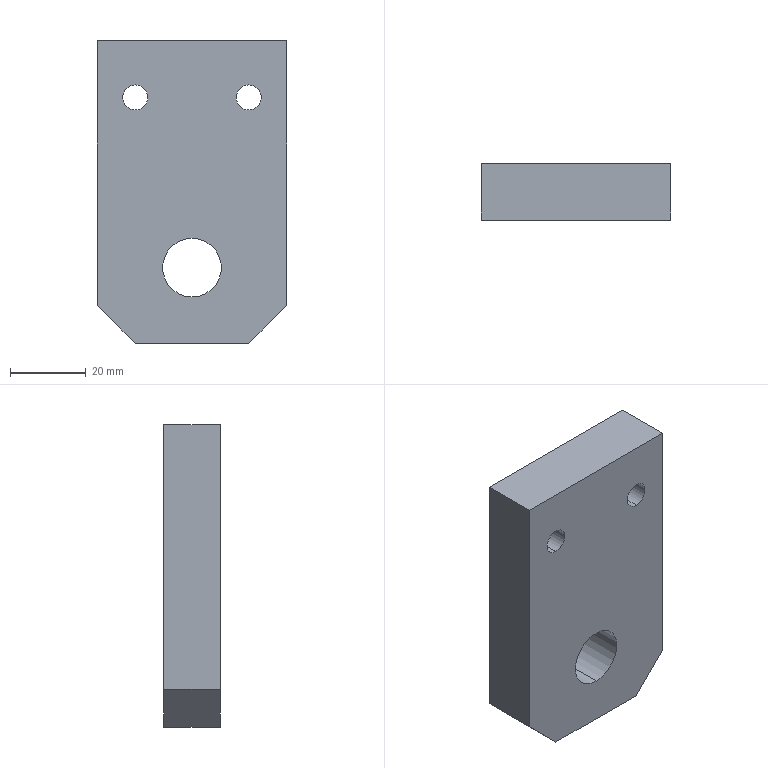Part | SolidWorks | features BaseBody 1 | 1 solid | 20 faces | box 50 x 15 x 80 mm | volume 53816 mm3 | cylinder 10 | plane 10 | commonest cylinder face diameters 6.6 x4 11 x4 15.5 x2
STEP:
#1=CARTESIAN_POINT('',(15.,8.2,-20.5));
#2=VERTEX_POINT('',#1);
#3=CARTESIAN_POINT('',(15.,8.2,-9.5));
#4=VERTEX_POINT('',#3);
#5=CARTESIAN_POINT('',(15.,8.2,-15.));
#6=DIRECTION('',(0.,1.,0.));
#7=DIRECTION('',(0.,0.,1.));
#8=AXIS2_PLACEMENT_3D('',#5,#6,#7);
#9=CIRCLE('',#8,5.5);
#10=EDGE_CURVE('',#2,#4,#9,.T.);
#11=ORIENTED_EDGE('',*,*,#10,.F.);
#12=CARTESIAN_POINT('',(15.,15.,-20.5));
#13=VERTEX_POINT('',#12);
#14=CARTESIAN_POINT('',(15.,15.,-20.5));
#15=DIRECTION('',(0.,1.,0.));
#16=VECTOR('',#15,1000.);
#17=LINE('',#14,#16);
#18=EDGE_CURVE('',#2,#13,#17,.T.);
#19=ORIENTED_EDGE('',*,*,#18,.T.);
#20=CARTESIAN_POINT('',(15.,15.,-9.5));
#21=VERTEX_POINT('',#20);
#22=CARTESIAN_POINT('',(15.,15.,-15.));
#23=DIRECTION('',(0.,1.,0.));
#24=DIRECTION('',(0.,0.,1.));
#25=AXIS2_PLACEMENT_3D('',#22,#23,#24);
#26=CIRCLE('',#25,5.5);
#27=EDGE_CURVE('',#13,#21,#26,.T.);
#28=ORIENTED_EDGE('',*,*,#27,.T.);
#29=CARTESIAN_POINT('',(15.,15.,-9.5));
#30=DIRECTION('',(0.,1.,0.));
#31=VECTOR('',#30,1000.);
#32=LINE('',#29,#31);
#33=EDGE_CURVE('',#4,#21,#32,.T.);
#34=ORIENTED_EDGE('',*,*,#33,.F.);
#35=EDGE_LOOP('',(#11,#19,#28,#34));
#36=FACE_OUTER_BOUND('',#35,.T.);
#37=CARTESIAN_POINT('',(15.,15.,-15.));
#38=DIRECTION('',(0.,1.,0.));
#39=DIRECTION('',(0.,0.,1.));
#40=AXIS2_PLACEMENT_3D('',#37,#38,#39);
#41=CYLINDRICAL_SURFACE('',#40,5.5);
#42=ADVANCED_FACE('',(#36),#41,.F.);
#43=CARTESIAN_POINT('',(15.,0.,-18.3));
#44=VERTEX_POINT('',#43);
#45=CARTESIAN_POINT('',(15.,0.,-11.7));
#46=VERTEX_POINT('',#45);
#47=CARTESIAN_POINT('',(15.,0.,-15.));
#48=DIRECTION('',(0.,1.,0.));
#49=DIRECTION('',(0.,0.,1.));
#50=AXIS2_PLACEMENT_3D('',#47,#48,#49);
#51=CIRCLE('',#50,3.3);
#52=EDGE_CURVE('',#44,#46,#51,.T.);
#53=ORIENTED_EDGE('',*,*,#52,.F.);
#54=CARTESIAN_POINT('',(15.,8.2,-18.3));
#55=VERTEX_POINT('',#54);
#56=CARTESIAN_POINT('',(15.,15.,-18.3));
#57=DIRECTION('',(0.,1.,0.));
#58=VECTOR('',#57,1000.);
#59=LINE('',#56,#58);
#60=EDGE_CURVE('',#44,#55,#59,.T.);
#61=ORIENTED_EDGE('',*,*,#60,.T.);
#62=CARTESIAN_POINT('',(15.,8.2,-11.7));
#63=VERTEX_POINT('',#62);
#64=CARTESIAN_POINT('',(15.,8.2,-15.));
#65=DIRECTION('',(0.,1.,0.));
#66=DIRECTION('',(0.,0.,1.));
#67=AXIS2_PLACEMENT_3D('',#64,#65,#66);
#68=CIRCLE('',#67,3.3);
#69=EDGE_CURVE('',#55,#63,#68,.T.);
#70=ORIENTED_EDGE('',*,*,#69,.T.);
#71=CARTESIAN_POINT('',(15.,15.,-11.7));
#72=DIRECTION('',(0.,1.,0.));
#73=VECTOR('',#72,1000.);
#74=LINE('',#71,#73);
#75=EDGE_CURVE('',#46,#63,#74,.T.);
#76=ORIENTED_EDGE('',*,*,#75,.F.);
#77=EDGE_LOOP('',(#53,#61,#70,#76));
#78=FACE_OUTER_BOUND('',#77,.T.);
#79=CARTESIAN_POINT('',(15.,15.,-15.));
#80=DIRECTION('',(0.,1.,0.));
#81=DIRECTION('',(0.,0.,1.));
#82=AXIS2_PLACEMENT_3D('',#79,#80,#81);
#83=CYLINDRICAL_SURFACE('',#82,3.3);
#84=ADVANCED_FACE('',(#78),#83,.F.);
#85=CARTESIAN_POINT('',(-15.,8.2,-20.5));
#86=VERTEX_POINT('',#85);
#87=CARTESIAN_POINT('',(-15.,8.2,-9.5));
#88=VERTEX_POINT('',#87);
#89=CARTESIAN_POINT('',(-15.,8.2,-15.));
#90=DIRECTION('',(0.,1.,0.));
#91=DIRECTION('',(0.,0.,1.));
#92=AXIS2_PLACEMENT_3D('',#89,#90,#91);
#93=CIRCLE('',#92,5.5);
#94=EDGE_CURVE('',#86,#88,#93,.T.);
#95=ORIENTED_EDGE('',*,*,#94,.F.);
#96=CARTESIAN_POINT('',(-15.,15.,-20.5));
#97=VERTEX_POINT('',#96);
#98=CARTESIAN_POINT('',(-15.,15.,-20.5));
#99=DIRECTION('',(0.,1.,0.));
#100=VECTOR('',#99,1000.);
#101=LINE('',#98,#100);
#102=EDGE_CURVE('',#86,#97,#101,.T.);
#103=ORIENTED_EDGE('',*,*,#102,.T.);
#104=CARTESIAN_POINT('',(-15.,15.,-9.5));
#105=VERTEX_POINT('',#104);
#106=CARTESIAN_POINT('',(-15.,15.,-15.));
#107=DIRECTION('',(0.,1.,0.));
#108=DIRECTION('',(0.,0.,1.));
#109=AXIS2_PLACEMENT_3D('',#106,#107,#108);
#110=CIRCLE('',#109,5.5);
#111=EDGE_CURVE('',#97,#105,#110,.T.);
#112=ORIENTED_EDGE('',*,*,#111,.T.);
#113=CARTESIAN_POINT('',(-15.,15.,-9.5));
#114=DIRECTION('',(0.,1.,0.));
#115=VECTOR('',#114,1000.);
#116=LINE('',#113,#115);
#117=EDGE_CURVE('',#88,#105,#116,.T.);
#118=ORIENTED_EDGE('',*,*,#117,.F.);
#119=EDGE_LOOP('',(#95,#103,#112,#118));
#120=FACE_OUTER_BOUND('',#119,.T.);
#121=CARTESIAN_POINT('',(-15.,15.,-15.));
#122=DIRECTION('',(0.,1.,0.));
#123=DIRECTION('',(0.,0.,1.));
#124=AXIS2_PLACEMENT_3D('',#121,#122,#123);
#125=CYLINDRICAL_SURFACE('',#124,5.5);
#126=ADVANCED_FACE('',(#120),#125,.F.);
#127=CARTESIAN_POINT('',(-15.,0.,-18.3));
#128=VERTEX_POINT('',#127);
#129=CARTESIAN_POINT('',(-15.,0.,-11.7));
#130=VERTEX_POINT('',#129);
#131=CARTESIAN_POINT('',(-15.,0.,-15.));
#132=DIRECTION('',(0.,1.,0.));
#133=DIRECTION('',(0.,0.,1.));
#134=AXIS2_PLACEMENT_3D('',#131,#132,#133);
#135=CIRCLE('',#134,3.3);
#136=EDGE_CURVE('',#128,#130,#135,.T.);
#137=ORIENTED_EDGE('',*,*,#136,.F.);
#138=CARTESIAN_POINT('',(-15.,8.2,-18.3));
#139=VERTEX_POINT('',#138);
#140=CARTESIAN_POINT('',(-15.,15.,-18.3));
#141=DIRECTION('',(0.,1.,0.));
#142=VECTOR('',#141,1000.);
#143=LINE('',#140,#142);
#144=EDGE_CURVE('',#128,#139,#143,.T.);
#145=ORIENTED_EDGE('',*,*,#144,.T.);
#146=CARTESIAN_POINT('',(-15.,8.2,-11.7));
#147=VERTEX_POINT('',#146);
#148=CARTESIAN_POINT('',(-15.,8.2,-15.));
#149=DIRECTION('',(0.,1.,0.));
#150=DIRECTION('',(0.,0.,1.));
#151=AXIS2_PLACEMENT_3D('',#148,#149,#150);
#152=CIRCLE('',#151,3.3);
#153=EDGE_CURVE('',#139,#147,#152,.T.);
#154=ORIENTED_EDGE('',*,*,#153,.T.);
#155=CARTESIAN_POINT('',(-15.,15.,-11.7));
#156=DIRECTION('',(0.,1.,0.));
#157=VECTOR('',#156,1000.);
#158=LINE('',#155,#157);
#159=EDGE_CURVE('',#130,#147,#158,.T.);
#160=ORIENTED_EDGE('',*,*,#159,.F.);
#161=EDGE_LOOP('',(#137,#145,#154,#160));
#162=FACE_OUTER_BOUND('',#161,.T.);
#163=CARTESIAN_POINT('',(-15.,15.,-15.));
#164=DIRECTION('',(0.,1.,0.));
#165=DIRECTION('',(0.,0.,1.));
#166=AXIS2_PLACEMENT_3D('',#163,#164,#165);
#167=CYLINDRICAL_SURFACE('',#166,3.3);
#168=ADVANCED_FACE('',(#162),#167,.F.);
#169=CARTESIAN_POINT('',(0.,0.,-67.75));
#170=VERTEX_POINT('',#169);
#171=CARTESIAN_POINT('',(0.,0.,-52.25));
#172=VERTEX_POINT('',#171);
#173=CARTESIAN_POINT('',(0.,0.,-60.));
#174=DIRECTION('',(0.,1.,0.));
#175=DIRECTION('',(0.,0.,1.));
#176=AXIS2_PLACEMENT_3D('',#173,#174,#175);
#177=CIRCLE('',#176,7.75);
#178=EDGE_CURVE('',#170,#172,#177,.T.);
#179=ORIENTED_EDGE('',*,*,#178,.F.);
#180=CARTESIAN_POINT('',(0.,15.,-67.75));
#181=VERTEX_POINT('',#180);
#182=CARTESIAN_POINT('',(0.,15.,-67.75));
#183=DIRECTION('',(0.,1.,0.));
#184=VECTOR('',#183,1000.);
#185=LINE('',#182,#184);
#186=EDGE_CURVE('',#170,#181,#185,.T.);
#187=ORIENTED_EDGE('',*,*,#186,.T.);
#188=CARTESIAN_POINT('',(0.,15.,-52.25));
#189=VERTEX_POINT('',#188);
#190=CARTESIAN_POINT('',(0.,15.,-60.));
#191=DIRECTION('',(0.,1.,0.));
#192=DIRECTION('',(0.,0.,1.));
#193=AXIS2_PLACEMENT_3D('',#190,#191,#192);
#194=CIRCLE('',#193,7.75);
#195=EDGE_CURVE('',#181,#189,#194,.T.);
#196=ORIENTED_EDGE('',*,*,#195,.T.);
#197=CARTESIAN_POINT('',(0.,15.,-52.25));
#198=DIRECTION('',(0.,1.,0.));
#199=VECTOR('',#198,1000.);
#200=LINE('',#197,#199);
#201=EDGE_CURVE('',#172,#189,#200,.T.);
#202=ORIENTED_EDGE('',*,*,#201,.F.);
#203=EDGE_LOOP('',(#179,#187,#196,#202));
#204=FACE_OUTER_BOUND('',#203,.T.);
#205=CARTESIAN_POINT('',(0.,15.,-60.));
#206=DIRECTION('',(0.,1.,0.));
#207=DIRECTION('',(0.,0.,1.));
#208=AXIS2_PLACEMENT_3D('',#205,#206,#207);
#209=CYLINDRICAL_SURFACE('',#208,7.75);
#210=ADVANCED_FACE('',(#204),#209,.F.);
#211=CARTESIAN_POINT('',(15.,8.2,-15.));
#212=DIRECTION('',(0.,1.,0.));
#213=DIRECTION('',(0.,0.,1.));
#214=AXIS2_PLACEMENT_3D('',#211,#212,#213);
#215=CIRCLE('',#214,3.3);
#216=EDGE_CURVE('',#63,#55,#215,.T.);
#217=ORIENTED_EDGE('',*,*,#216,.F.);
#218=ORIENTED_EDGE('',*,*,#69,.F.);
#219=EDGE_LOOP('',(#217,#218));
#220=FACE_BOUND('',#219,.T.);
#221=CARTESIAN_POINT('',(15.,8.2,-15.));
#222=DIRECTION('',(0.,1.,0.));
#223=DIRECTION('',(0.,0.,1.));
#224=AXIS2_PLACEMENT_3D('',#221,#222,#223);
#225=CIRCLE('',#224,5.5);
#226=EDGE_CURVE('',#4,#2,#225,.T.);
#227=ORIENTED_EDGE('',*,*,#226,.T.);
#228=ORIENTED_EDGE('',*,*,#10,.T.);
#229=EDGE_LOOP('',(#227,#228));
#230=FACE_OUTER_BOUND('',#229,.T.);
#231=CARTESIAN_POINT('',(18.3,8.2,-15.));
#232=DIRECTION('',(0.,-1.,0.));
#233=DIRECTION('',(0.,0.,-1.));
#234=AXIS2_PLACEMENT_3D('',#231,#232,#233);
#235=PLANE('',#234);
#236=ADVANCED_FACE('',(#220,#230),#235,.F.);
#237=CARTESIAN_POINT('',(-15.,8.2,-15.));
#238=DIRECTION('',(0.,1.,0.));
#239=DIRECTION('',(0.,0.,1.));
#240=AXIS2_PLACEMENT_3D('',#237,#238,#239);
#241=CIRCLE('',#240,3.3);
#242=EDGE_CURVE('',#147,#139,#241,.T.);
#243=ORIENTED_EDGE('',*,*,#242,.F.);
#244=ORIENTED_EDGE('',*,*,#153,.F.);
#245=EDGE_LOOP('',(#243,#244));
#246=FACE_BOUND('',#245,.T.);
#247=CARTESIAN_POINT('',(-15.,8.2,-15.));
#248=DIRECTION('',(0.,1.,0.));
#249=DIRECTION('',(0.,0.,1.));
#250=AXIS2_PLACEMENT_3D('',#247,#248,#249);
#251=CIRCLE('',#250,5.5);
#252=EDGE_CURVE('',#88,#86,#251,.T.);
#253=ORIENTED_EDGE('',*,*,#252,.T.);
#254=ORIENTED_EDGE('',*,*,#94,.T.);
#255=EDGE_LOOP('',(#253,#254));
#256=FACE_OUTER_BOUND('',#255,.T.);
#257=CARTESIAN_POINT('',(-11.7,8.2,-15.));
#258=DIRECTION('',(0.,-1.,0.));
#259=DIRECTION('',(0.,0.,-1.));
#260=AXIS2_PLACEMENT_3D('',#257,#258,#259);
#261=PLANE('',#260);
#262=ADVANCED_FACE('',(#246,#256),#261,.F.);
#263=CARTESIAN_POINT('',(25.,15.,-70.));
#264=VERTEX_POINT('',#263);
#265=CARTESIAN_POINT('',(15.,15.,-80.));
#266=VERTEX_POINT('',#265);
#267=CARTESIAN_POINT('',(15.,15.,-80.));
#268=DIRECTION('',(-0.7071,0.,-0.7071));
#269=VECTOR('',#268,1000.);
#270=LINE('',#267,#269);
#271=EDGE_CURVE('',#264,#266,#270,.T.);
#272=ORIENTED_EDGE('',*,*,#271,.F.);
#273=CARTESIAN_POINT('',(25.,0.,-70.));
#274=VERTEX_POINT('',#273);
#275=CARTESIAN_POINT('',(25.,15.,-70.));
#276=DIRECTION('',(0.,1.,0.));
#277=VECTOR('',#276,1000.);
#278=LINE('',#275,#277);
#279=EDGE_CURVE('',#274,#264,#278,.T.);
#280=ORIENTED_EDGE('',*,*,#279,.F.);
#281=CARTESIAN_POINT('',(15.,0.,-80.));
#282=VERTEX_POINT('',#281);
#283=CARTESIAN_POINT('',(47.5,0.,-47.5));
#284=DIRECTION('',(0.7071,0.,0.7071));
#285=VECTOR('',#284,1000.);
#286=LINE('',#283,#285);
#287=EDGE_CURVE('',#282,#274,#286,.T.);
#288=ORIENTED_EDGE('',*,*,#287,.F.);
#289=CARTESIAN_POINT('',(15.,15.,-80.));
#290=DIRECTION('',(0.,-1.,0.));
#291=VECTOR('',#290,1000.);
#292=LINE('',#289,#291);
#293=EDGE_CURVE('',#266,#282,#292,.T.);
#294=ORIENTED_EDGE('',*,*,#293,.F.);
#295=EDGE_LOOP('',(#272,#280,#288,#294));
#296=FACE_OUTER_BOUND('',#295,.T.);
#297=CARTESIAN_POINT('',(15.,15.,-80.));
#298=DIRECTION('',(-0.7071,0.,0.7071));
#299=DIRECTION('',(0.,1.,0.));
#300=AXIS2_PLACEMENT_3D('',#297,#298,#299);
#301=PLANE('',#300);
#302=ADVANCED_FACE('',(#296),#301,.F.);
#303=CARTESIAN_POINT('',(-15.,15.,-80.));
#304=VERTEX_POINT('',#303);
#305=CARTESIAN_POINT('',(-25.,15.,-70.));
#306=VERTEX_POINT('',#305);
#307=CARTESIAN_POINT('',(-25.,15.,-70.));
#308=DIRECTION('',(-0.7071,0.,0.7071));
#309=VECTOR('',#308,1000.);
#310=LINE('',#307,#309);
#311=EDGE_CURVE('',#304,#306,#310,.T.);
#312=ORIENTED_EDGE('',*,*,#311,.F.);
#313=CARTESIAN_POINT('',(-15.,0.,-80.));
#314=VERTEX_POINT('',#313);
#315=CARTESIAN_POINT('',(-15.,15.,-80.));
#316=DIRECTION('',(0.,1.,0.));
#317=VECTOR('',#316,1000.);
#318=LINE('',#315,#317);
#319=EDGE_CURVE('',#314,#304,#318,.T.);
#320=ORIENTED_EDGE('',*,*,#319,.F.);
#321=CARTESIAN_POINT('',(-25.,0.,-70.));
#322=VERTEX_POINT('',#321);
#323=CARTESIAN_POINT('',(-47.5,0.,-47.5));
#324=DIRECTION('',(0.7071,0.,-0.7071));
#325=VECTOR('',#324,1000.);
#326=LINE('',#323,#325);
#327=EDGE_CURVE('',#322,#314,#326,.T.);
#328=ORIENTED_EDGE('',*,*,#327,.F.);
#329=CARTESIAN_POINT('',(-25.,15.,-70.));
#330=DIRECTION('',(0.,-1.,0.));
#331=VECTOR('',#330,1000.);
#332=LINE('',#329,#331);
#333=EDGE_CURVE('',#306,#322,#332,.T.);
#334=ORIENTED_EDGE('',*,*,#333,.F.);
#335=EDGE_LOOP('',(#312,#320,#328,#334));
#336=FACE_OUTER_BOUND('',#335,.T.);
#337=CARTESIAN_POINT('',(-25.,15.,-70.));
#338=DIRECTION('',(0.7071,0.,0.7071));
#339=DIRECTION('',(0.,-1.,0.));
#340=AXIS2_PLACEMENT_3D('',#337,#338,#339);
#341=PLANE('',#340);
#342=ADVANCED_FACE('',(#336),#341,.F.);
#343=CARTESIAN_POINT('',(0.,0.,-60.));
#344=DIRECTION('',(0.,1.,0.));
#345=DIRECTION('',(0.,0.,1.));
#346=AXIS2_PLACEMENT_3D('',#343,#344,#345);
#347=CIRCLE('',#346,7.75);
#348=EDGE_CURVE('',#172,#170,#347,.T.);
#349=ORIENTED_EDGE('',*,*,#348,.T.);
#350=ORIENTED_EDGE('',*,*,#178,.T.);
#351=EDGE_LOOP('',(#349,#350));
#352=FACE_BOUND('',#351,.T.);
#353=CARTESIAN_POINT('',(-15.,0.,-15.));
#354=DIRECTION('',(0.,1.,0.));
#355=DIRECTION('',(0.,0.,1.));
#356=AXIS2_PLACEMENT_3D('',#353,#354,#355);
#357=CIRCLE('',#356,3.3);
#358=EDGE_CURVE('',#130,#128,#357,.T.);
#359=ORIENTED_EDGE('',*,*,#358,.T.);
#360=ORIENTED_EDGE('',*,*,#136,.T.);
#361=EDGE_LOOP('',(#359,#360));
#362=FACE_BOUND('',#361,.T.);
#363=CARTESIAN_POINT('',(15.,0.,-15.));
#364=DIRECTION('',(0.,1.,0.));
#365=DIRECTION('',(0.,0.,1.));
#366=AXIS2_PLACEMENT_3D('',#363,#364,#365);
#367=CIRCLE('',#366,3.3);
#368=EDGE_CURVE('',#46,#44,#367,.T.);
#369=ORIENTED_EDGE('',*,*,#368,.T.);
#370=ORIENTED_EDGE('',*,*,#52,.T.);
#371=EDGE_LOOP('',(#369,#370));
#372=FACE_BOUND('',#371,.T.);
#373=CARTESIAN_POINT('',(-25.,0.,0.));
#374=VERTEX_POINT('',#373);
#375=CARTESIAN_POINT('',(-25.,0.,0.));
#376=DIRECTION('',(0.,0.,1.));
#377=VECTOR('',#376,1000.);
#378=LINE('',#375,#377);
#379=EDGE_CURVE('',#322,#374,#378,.T.);
#380=ORIENTED_EDGE('',*,*,#379,.F.);
#381=ORIENTED_EDGE('',*,*,#327,.T.);
#382=CARTESIAN_POINT('',(-25.,0.,-80.));
#383=DIRECTION('',(-1.,0.,0.));
#384=VECTOR('',#383,1000.);
#385=LINE('',#382,#384);
#386=EDGE_CURVE('',#282,#314,#385,.T.);
#387=ORIENTED_EDGE('',*,*,#386,.F.);
#388=ORIENTED_EDGE('',*,*,#287,.T.);
#389=CARTESIAN_POINT('',(25.,0.,0.));
#390=VERTEX_POINT('',#389);
#391=CARTESIAN_POINT('',(25.,0.,0.));
#392=DIRECTION('',(0.,0.,-1.));
#393=VECTOR('',#392,1000.);
#394=LINE('',#391,#393);
#395=EDGE_CURVE('',#390,#274,#394,.T.);
#396=ORIENTED_EDGE('',*,*,#395,.F.);
#397=CARTESIAN_POINT('',(-25.,0.,0.));
#398=DIRECTION('',(1.,0.,0.));
#399=VECTOR('',#398,1000.);
#400=LINE('',#397,#399);
#401=EDGE_CURVE('',#374,#390,#400,.T.);
#402=ORIENTED_EDGE('',*,*,#401,.F.);
#403=EDGE_LOOP('',(#380,#381,#387,#388,#396,#402));
#404=FACE_OUTER_BOUND('',#403,.T.);
#405=CARTESIAN_POINT('',(0.,0.,0.));
#406=DIRECTION('',(0.,-1.,0.));
#407=DIRECTION('',(0.,0.,-1.));
#408=AXIS2_PLACEMENT_3D('',#405,#406,#407);
#409=PLANE('',#408);
#410=ADVANCED_FACE('',(#352,#362,#372,#404),#409,.T.);
#411=CARTESIAN_POINT('',(0.,15.,-60.));
#412=DIRECTION('',(0.,1.,0.));
#413=DIRECTION('',(0.,0.,1.));
#414=AXIS2_PLACEMENT_3D('',#411,#412,#413);
#415=CIRCLE('',#414,7.75);
#416=EDGE_CURVE('',#189,#181,#415,.T.);
#417=ORIENTED_EDGE('',*,*,#416,.F.);
#418=ORIENTED_EDGE('',*,*,#195,.F.);
#419=EDGE_LOOP('',(#417,#418));
#420=FACE_BOUND('',#419,.T.);
#421=CARTESIAN_POINT('',(-15.,15.,-15.));
#422=DIRECTION('',(0.,1.,0.));
#423=DIRECTION('',(0.,0.,1.));
#424=AXIS2_PLACEMENT_3D('',#421,#422,#423);
#425=CIRCLE('',#424,5.5);
#426=EDGE_CURVE('',#105,#97,#425,.T.);
#427=ORIENTED_EDGE('',*,*,#426,.F.);
#428=ORIENTED_EDGE('',*,*,#111,.F.);
#429=EDGE_LOOP('',(#427,#428));
#430=FACE_BOUND('',#429,.T.);
#431=CARTESIAN_POINT('',(15.,15.,-15.));
#432=DIRECTION('',(0.,1.,0.));
#433=DIRECTION('',(0.,0.,1.));
#434=AXIS2_PLACEMENT_3D('',#431,#432,#433);
#435=CIRCLE('',#434,5.5);
#436=EDGE_CURVE('',#21,#13,#435,.T.);
#437=ORIENTED_EDGE('',*,*,#436,.F.);
#438=ORIENTED_EDGE('',*,*,#27,.F.);
#439=EDGE_LOOP('',(#437,#438));
#440=FACE_BOUND('',#439,.T.);
#441=CARTESIAN_POINT('',(-25.,15.,-80.));
#442=DIRECTION('',(-1.,0.,0.));
#443=VECTOR('',#442,1000.);
#444=LINE('',#441,#443);
#445=EDGE_CURVE('',#266,#304,#444,.T.);
#446=ORIENTED_EDGE('',*,*,#445,.T.);
#447=ORIENTED_EDGE('',*,*,#311,.T.);
#448=CARTESIAN_POINT('',(-25.,15.,0.));
#449=VERTEX_POINT('',#448);
#450=CARTESIAN_POINT('',(-25.,15.,0.));
#451=DIRECTION('',(0.,0.,1.));
#452=VECTOR('',#451,1000.);
#453=LINE('',#450,#452);
#454=EDGE_CURVE('',#306,#449,#453,.T.);
#455=ORIENTED_EDGE('',*,*,#454,.T.);
#456=CARTESIAN_POINT('',(25.,15.,0.));
#457=VERTEX_POINT('',#456);
#458=CARTESIAN_POINT('',(-25.,15.,0.));
#459=DIRECTION('',(1.,0.,0.));
#460=VECTOR('',#459,1000.);
#461=LINE('',#458,#460);
#462=EDGE_CURVE('',#449,#457,#461,.T.);
#463=ORIENTED_EDGE('',*,*,#462,.T.);
#464=CARTESIAN_POINT('',(25.,15.,0.));
#465=DIRECTION('',(0.,0.,-1.));
#466=VECTOR('',#465,1000.);
#467=LINE('',#464,#466);
#468=EDGE_CURVE('',#457,#264,#467,.T.);
#469=ORIENTED_EDGE('',*,*,#468,.T.);
#470=ORIENTED_EDGE('',*,*,#271,.T.);
#471=EDGE_LOOP('',(#446,#447,#455,#463,#469,#470));
#472=FACE_OUTER_BOUND('',#471,.T.);
#473=CARTESIAN_POINT('',(0.,15.,0.));
#474=DIRECTION('',(0.,-1.,0.));
#475=DIRECTION('',(0.,0.,-1.));
#476=AXIS2_PLACEMENT_3D('',#473,#474,#475);
#477=PLANE('',#476);
#478=ADVANCED_FACE('',(#420,#430,#440,#472),#477,.F.);
#479=ORIENTED_EDGE('',*,*,#386,.T.);
#480=ORIENTED_EDGE('',*,*,#319,.T.);
#481=ORIENTED_EDGE('',*,*,#445,.F.);
#482=ORIENTED_EDGE('',*,*,#293,.T.);
#483=EDGE_LOOP('',(#479,#480,#481,#482));
#484=FACE_OUTER_BOUND('',#483,.T.);
#485=CARTESIAN_POINT('',(-25.,15.,-80.));
#486=DIRECTION('',(0.,0.,1.));
#487=DIRECTION('',(1.,0.,0.));
#488=AXIS2_PLACEMENT_3D('',#485,#486,#487);
#489=PLANE('',#488);
#490=ADVANCED_FACE('',(#484),#489,.F.);
#491=ORIENTED_EDGE('',*,*,#395,.T.);
#492=ORIENTED_EDGE('',*,*,#279,.T.);
#493=ORIENTED_EDGE('',*,*,#468,.F.);
#494=CARTESIAN_POINT('',(25.,15.,0.));
#495=DIRECTION('',(0.,-1.,0.));
#496=VECTOR('',#495,1000.);
#497=LINE('',#494,#496);
#498=EDGE_CURVE('',#457,#390,#497,.T.);
#499=ORIENTED_EDGE('',*,*,#498,.T.);
#500=EDGE_LOOP('',(#491,#492,#493,#499));
#501=FACE_OUTER_BOUND('',#500,.T.);
#502=CARTESIAN_POINT('',(25.,15.,0.));
#503=DIRECTION('',(-1.,0.,0.));
#504=DIRECTION('',(0.,0.,1.));
#505=AXIS2_PLACEMENT_3D('',#502,#503,#504);
#506=PLANE('',#505);
#507=ADVANCED_FACE('',(#501),#506,.F.);
#508=ORIENTED_EDGE('',*,*,#401,.T.);
#509=ORIENTED_EDGE('',*,*,#498,.F.);
#510=ORIENTED_EDGE('',*,*,#462,.F.);
#511=CARTESIAN_POINT('',(-25.,15.,0.));
#512=DIRECTION('',(0.,-1.,0.));
#513=VECTOR('',#512,1000.);
#514=LINE('',#511,#513);
#515=EDGE_CURVE('',#449,#374,#514,.T.);
#516=ORIENTED_EDGE('',*,*,#515,.T.);
#517=EDGE_LOOP('',(#508,#509,#510,#516));
#518=FACE_OUTER_BOUND('',#517,.T.);
#519=CARTESIAN_POINT('',(-25.,15.,0.));
#520=DIRECTION('',(0.,0.,-1.));
#521=DIRECTION('',(0.,-1.,0.));
#522=AXIS2_PLACEMENT_3D('',#519,#520,#521);
#523=PLANE('',#522);
#524=ADVANCED_FACE('',(#518),#523,.F.);
#525=ORIENTED_EDGE('',*,*,#454,.F.);
#526=ORIENTED_EDGE('',*,*,#333,.T.);
#527=ORIENTED_EDGE('',*,*,#379,.T.);
#528=ORIENTED_EDGE('',*,*,#515,.F.);
#529=EDGE_LOOP('',(#525,#526,#527,#528));
#530=FACE_OUTER_BOUND('',#529,.T.);
#531=CARTESIAN_POINT('',(-25.,15.,0.));
#532=DIRECTION('',(1.,0.,0.));
#533=DIRECTION('',(0.,1.,0.));
#534=AXIS2_PLACEMENT_3D('',#531,#532,#533);
#535=PLANE('',#534);
#536=ADVANCED_FACE('',(#530),#535,.F.);
#537=ORIENTED_EDGE('',*,*,#186,.F.);
#538=ORIENTED_EDGE('',*,*,#348,.F.);
#539=ORIENTED_EDGE('',*,*,#201,.T.);
#540=ORIENTED_EDGE('',*,*,#416,.T.);
#541=EDGE_LOOP('',(#537,#538,#539,#540));
#542=FACE_OUTER_BOUND('',#541,.T.);
#543=CARTESIAN_POINT('',(0.,15.,-60.));
#544=DIRECTION('',(0.,1.,0.));
#545=DIRECTION('',(0.,0.,1.));
#546=AXIS2_PLACEMENT_3D('',#543,#544,#545);
#547=CYLINDRICAL_SURFACE('',#546,7.75);
#548=ADVANCED_FACE('',(#542),#547,.F.);
#549=ORIENTED_EDGE('',*,*,#144,.F.);
#550=ORIENTED_EDGE('',*,*,#358,.F.);
#551=ORIENTED_EDGE('',*,*,#159,.T.);
#552=ORIENTED_EDGE('',*,*,#242,.T.);
#553=EDGE_LOOP('',(#549,#550,#551,#552));
#554=FACE_OUTER_BOUND('',#553,.T.);
#555=CARTESIAN_POINT('',(-15.,15.,-15.));
#556=DIRECTION('',(0.,1.,0.));
#557=DIRECTION('',(0.,0.,1.));
#558=AXIS2_PLACEMENT_3D('',#555,#556,#557);
#559=CYLINDRICAL_SURFACE('',#558,3.3);
#560=ADVANCED_FACE('',(#554),#559,.F.);
#561=ORIENTED_EDGE('',*,*,#102,.F.);
#562=ORIENTED_EDGE('',*,*,#252,.F.);
#563=ORIENTED_EDGE('',*,*,#117,.T.);
#564=ORIENTED_EDGE('',*,*,#426,.T.);
#565=EDGE_LOOP('',(#561,#562,#563,#564));
#566=FACE_OUTER_BOUND('',#565,.T.);
#567=CARTESIAN_POINT('',(-15.,15.,-15.));
#568=DIRECTION('',(0.,1.,0.));
#569=DIRECTION('',(0.,0.,1.));
#570=AXIS2_PLACEMENT_3D('',#567,#568,#569);
#571=CYLINDRICAL_SURFACE('',#570,5.5);
#572=ADVANCED_FACE('',(#566),#571,.F.);
#573=ORIENTED_EDGE('',*,*,#60,.F.);
#574=ORIENTED_EDGE('',*,*,#368,.F.);
#575=ORIENTED_EDGE('',*,*,#75,.T.);
#576=ORIENTED_EDGE('',*,*,#216,.T.);
#577=EDGE_LOOP('',(#573,#574,#575,#576));
#578=FACE_OUTER_BOUND('',#577,.T.);
#579=CARTESIAN_POINT('',(15.,15.,-15.));
#580=DIRECTION('',(0.,1.,0.));
#581=DIRECTION('',(0.,0.,1.));
#582=AXIS2_PLACEMENT_3D('',#579,#580,#581);
#583=CYLINDRICAL_SURFACE('',#582,3.3);
#584=ADVANCED_FACE('',(#578),#583,.F.);
#585=ORIENTED_EDGE('',*,*,#18,.F.);
#586=ORIENTED_EDGE('',*,*,#226,.F.);
#587=ORIENTED_EDGE('',*,*,#33,.T.);
#588=ORIENTED_EDGE('',*,*,#436,.T.);
#589=EDGE_LOOP('',(#585,#586,#587,#588));
#590=FACE_OUTER_BOUND('',#589,.T.);
#591=CARTESIAN_POINT('',(15.,15.,-15.));
#592=DIRECTION('',(0.,1.,0.));
#593=DIRECTION('',(0.,0.,1.));
#594=AXIS2_PLACEMENT_3D('',#591,#592,#593);
#595=CYLINDRICAL_SURFACE('',#594,5.5);
#596=ADVANCED_FACE('',(#590),#595,.F.);
#597=CLOSED_SHELL('',(#42,#84,#126,#168,#210,#236,#262,#302,#342,#410,#478,#490,#507,#524,#536,#548,#560,#572,#584,#596));
#598=MANIFOLD_SOLID_BREP('',#597);
#599=CARTESIAN_POINT('',(0.,0.,0.));
#600=DIRECTION('',(0.,0.,1.));
#601=DIRECTION('',(1.,0.,0.));
#602=AXIS2_PLACEMENT_3D('',#599,#600,#601);
#603=(LENGTH_UNIT()NAMED_UNIT(*)SI_UNIT(.MILLI.,.METRE.));
#604=UNCERTAINTY_MEASURE_WITH_UNIT(LENGTH_MEASURE(0.00001),#603,'','');
#605=(NAMED_UNIT(*)PLANE_ANGLE_UNIT()SI_UNIT($,.RADIAN.));
#606=(NAMED_UNIT(*)SI_UNIT($,.STERADIAN.)SOLID_ANGLE_UNIT());
#607=(GEOMETRIC_REPRESENTATION_CONTEXT(3)GLOBAL_UNCERTAINTY_ASSIGNED_CONTEXT((#604))GLOBAL_UNIT_ASSIGNED_CONTEXT((#603,#605,#606))REPRESENTATION_CONTEXT('',''));
#608=ADVANCED_BREP_SHAPE_REPRESENTATION('',(#598,#602),#607);